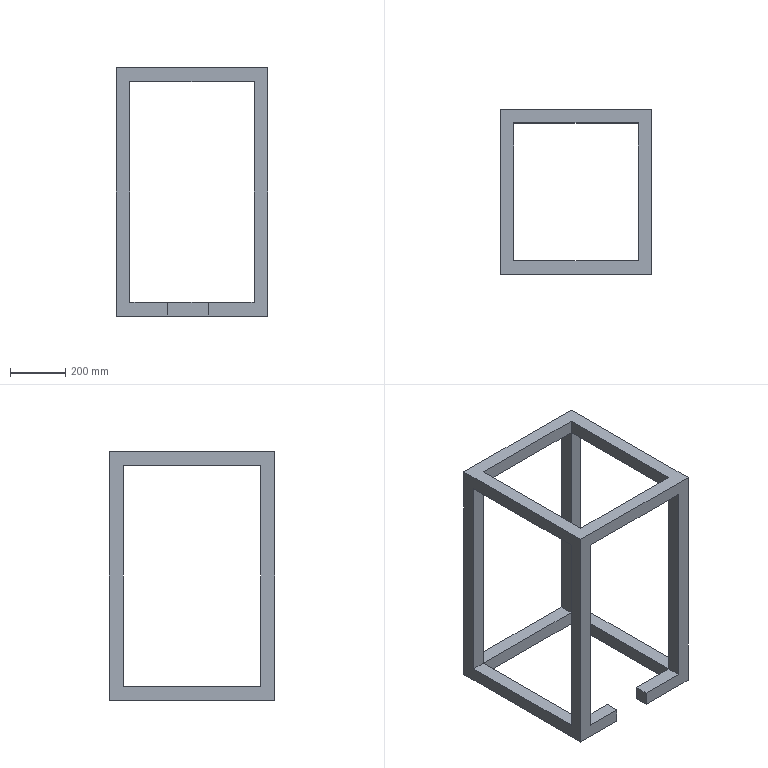Part | STEP file | frame | 1 solid | 34 faces | box 550 x 600 x 900 mm | volume 18125000 mm3 | plane 34